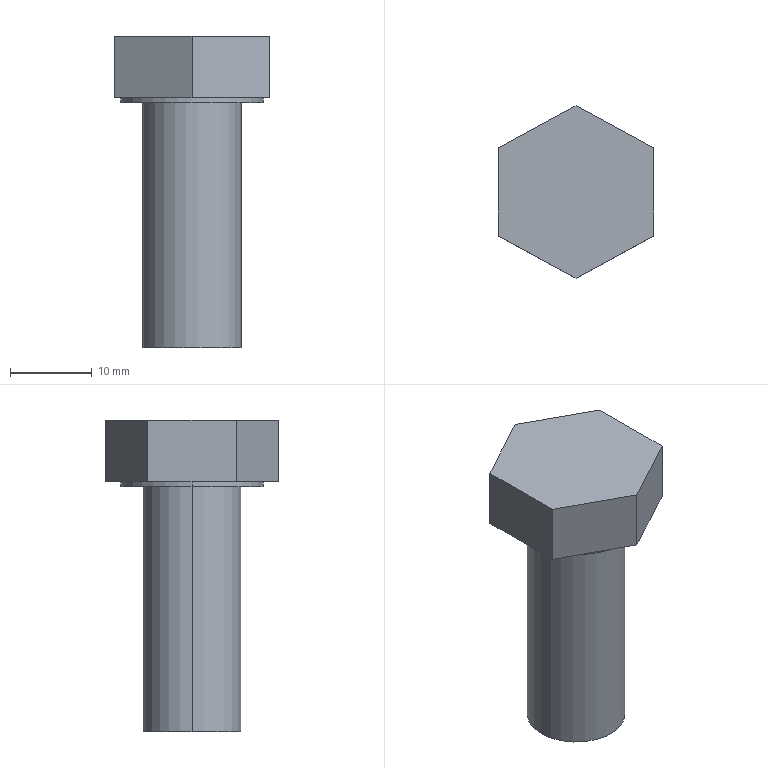Part | STEP file | M12-30 | 1 solid | 14 faces | box 19 x 21.1 x 38.1 mm | volume 5809 mm3 | plane 10 | cylinder 4 | commonest cylinder face diameters 12 x2 17.4 x2
STEP:
#1=CARTESIAN_POINT('',(0.,0.,0.));
#2=DIRECTION('',(0.,0.,1.));
#3=DIRECTION('',(1.,0.,0.));
#4=AXIS2_PLACEMENT_3D('',#1,#2,#3);
#5=CARTESIAN_POINT('',(0.,10.55,0.));
#6=VERTEX_POINT('',#5);
#7=CARTESIAN_POINT('',(-9.5,5.402,0.));
#8=VERTEX_POINT('',#7);
#9=CARTESIAN_POINT('',(0.,10.55,0.));
#10=DIRECTION('',(-0.8792,-0.4764,0.));
#11=VECTOR('',#10,1.);
#12=LINE('',#9,#11);
#13=CARTESIAN_POINT('',(0.,0.,0.));
#14=DIRECTION('',(0.,0.,1.));
#15=DIRECTION('',(1.,0.,0.));
#16=AXIS2_PLACEMENT_3D('',#13,#14,#15);
#17=PLANE('',#16);
#18=CARTESIAN_POINT('',(0.,10.55));
#19=DIRECTION('',(-0.8792,-0.4764));
#20=VECTOR('',#19,1.);
#21=LINE('',#18,#20);
#22=(GEOMETRIC_REPRESENTATION_CONTEXT(2)PARAMETRIC_REPRESENTATION_CONTEXT()REPRESENTATION_CONTEXT('',''));
#23=DEFINITIONAL_REPRESENTATION('',(#21),#22);
#24=PCURVE('',#17,#23);
#25=CARTESIAN_POINT('',(0.,10.55,0.));
#26=DIRECTION('',(-0.4764,0.8792,0.));
#27=DIRECTION('',(-0.8792,-0.4764,0.));
#28=AXIS2_PLACEMENT_3D('',#25,#26,#27);
#29=PLANE('',#28);
#30=CARTESIAN_POINT('',(0.,0.));
#31=DIRECTION('',(1.,0.));
#32=VECTOR('',#31,1.);
#33=LINE('',#30,#32);
#34=(GEOMETRIC_REPRESENTATION_CONTEXT(2)PARAMETRIC_REPRESENTATION_CONTEXT()REPRESENTATION_CONTEXT('',''));
#35=DEFINITIONAL_REPRESENTATION('',(#33),#34);
#36=PCURVE('',#29,#35);
#37=SURFACE_CURVE('',#12,(#24,#36),.PCURVE_S1.);
#38=EDGE_CURVE('',#6,#8,#37,.T.);
#39=ORIENTED_EDGE('',*,*,#38,.T.);
#40=CARTESIAN_POINT('',(-9.5,-5.402,0.));
#41=VERTEX_POINT('',#40);
#42=CARTESIAN_POINT('',(-9.5,5.402,0.));
#43=DIRECTION('',(0.,-1.,0.));
#44=VECTOR('',#43,1.);
#45=LINE('',#42,#44);
#46=CARTESIAN_POINT('',(-9.5,5.402));
#47=DIRECTION('',(0.,-1.));
#48=VECTOR('',#47,1.);
#49=LINE('',#46,#48);
#50=(GEOMETRIC_REPRESENTATION_CONTEXT(2)PARAMETRIC_REPRESENTATION_CONTEXT()REPRESENTATION_CONTEXT('',''));
#51=DEFINITIONAL_REPRESENTATION('',(#49),#50);
#52=PCURVE('',#17,#51);
#53=CARTESIAN_POINT('',(-9.5,5.402,0.));
#54=DIRECTION('',(-1.,0.,0.));
#55=DIRECTION('',(0.,-1.,0.));
#56=AXIS2_PLACEMENT_3D('',#53,#54,#55);
#57=PLANE('',#56);
#58=CARTESIAN_POINT('',(0.,0.));
#59=DIRECTION('',(1.,0.));
#60=VECTOR('',#59,1.);
#61=LINE('',#58,#60);
#62=(GEOMETRIC_REPRESENTATION_CONTEXT(2)PARAMETRIC_REPRESENTATION_CONTEXT()REPRESENTATION_CONTEXT('',''));
#63=DEFINITIONAL_REPRESENTATION('',(#61),#62);
#64=PCURVE('',#57,#63);
#65=SURFACE_CURVE('',#45,(#52,#64),.PCURVE_S1.);
#66=EDGE_CURVE('',#8,#41,#65,.T.);
#67=ORIENTED_EDGE('',*,*,#66,.T.);
#68=CARTESIAN_POINT('',(0.,-10.55,0.));
#69=VERTEX_POINT('',#68);
#70=CARTESIAN_POINT('',(-9.5,-5.402,0.));
#71=DIRECTION('',(0.8792,-0.4764,0.));
#72=VECTOR('',#71,1.);
#73=LINE('',#70,#72);
#74=CARTESIAN_POINT('',(-9.5,-5.402));
#75=DIRECTION('',(0.8792,-0.4764));
#76=VECTOR('',#75,1.);
#77=LINE('',#74,#76);
#78=(GEOMETRIC_REPRESENTATION_CONTEXT(2)PARAMETRIC_REPRESENTATION_CONTEXT()REPRESENTATION_CONTEXT('',''));
#79=DEFINITIONAL_REPRESENTATION('',(#77),#78);
#80=PCURVE('',#17,#79);
#81=CARTESIAN_POINT('',(-9.5,-5.402,0.));
#82=DIRECTION('',(-0.4764,-0.8792,0.));
#83=DIRECTION('',(0.8792,-0.4764,0.));
#84=AXIS2_PLACEMENT_3D('',#81,#82,#83);
#85=PLANE('',#84);
#86=CARTESIAN_POINT('',(0.,0.));
#87=DIRECTION('',(1.,0.));
#88=VECTOR('',#87,1.);
#89=LINE('',#86,#88);
#90=(GEOMETRIC_REPRESENTATION_CONTEXT(2)PARAMETRIC_REPRESENTATION_CONTEXT()REPRESENTATION_CONTEXT('',''));
#91=DEFINITIONAL_REPRESENTATION('',(#89),#90);
#92=PCURVE('',#85,#91);
#93=SURFACE_CURVE('',#73,(#80,#92),.PCURVE_S1.);
#94=EDGE_CURVE('',#41,#69,#93,.T.);
#95=ORIENTED_EDGE('',*,*,#94,.T.);
#96=CARTESIAN_POINT('',(9.5,-5.402,0.));
#97=VERTEX_POINT('',#96);
#98=CARTESIAN_POINT('',(0.,-10.55,0.));
#99=DIRECTION('',(0.8792,0.4764,0.));
#100=VECTOR('',#99,1.);
#101=LINE('',#98,#100);
#102=CARTESIAN_POINT('',(0.,-10.55));
#103=DIRECTION('',(0.8792,0.4764));
#104=VECTOR('',#103,1.);
#105=LINE('',#102,#104);
#106=(GEOMETRIC_REPRESENTATION_CONTEXT(2)PARAMETRIC_REPRESENTATION_CONTEXT()REPRESENTATION_CONTEXT('',''));
#107=DEFINITIONAL_REPRESENTATION('',(#105),#106);
#108=PCURVE('',#17,#107);
#109=CARTESIAN_POINT('',(0.,-10.55,0.));
#110=DIRECTION('',(0.4764,-0.8792,0.));
#111=DIRECTION('',(0.8792,0.4764,0.));
#112=AXIS2_PLACEMENT_3D('',#109,#110,#111);
#113=PLANE('',#112);
#114=CARTESIAN_POINT('',(0.,0.));
#115=DIRECTION('',(1.,0.));
#116=VECTOR('',#115,1.);
#117=LINE('',#114,#116);
#118=(GEOMETRIC_REPRESENTATION_CONTEXT(2)PARAMETRIC_REPRESENTATION_CONTEXT()REPRESENTATION_CONTEXT('',''));
#119=DEFINITIONAL_REPRESENTATION('',(#117),#118);
#120=PCURVE('',#113,#119);
#121=SURFACE_CURVE('',#101,(#108,#120),.PCURVE_S1.);
#122=EDGE_CURVE('',#69,#97,#121,.T.);
#123=ORIENTED_EDGE('',*,*,#122,.T.);
#124=CARTESIAN_POINT('',(9.5,5.402,0.));
#125=VERTEX_POINT('',#124);
#126=CARTESIAN_POINT('',(9.5,-5.402,0.));
#127=DIRECTION('',(0.,1.,0.));
#128=VECTOR('',#127,1.);
#129=LINE('',#126,#128);
#130=CARTESIAN_POINT('',(9.5,-5.402));
#131=DIRECTION('',(0.,1.));
#132=VECTOR('',#131,1.);
#133=LINE('',#130,#132);
#134=(GEOMETRIC_REPRESENTATION_CONTEXT(2)PARAMETRIC_REPRESENTATION_CONTEXT()REPRESENTATION_CONTEXT('',''));
#135=DEFINITIONAL_REPRESENTATION('',(#133),#134);
#136=PCURVE('',#17,#135);
#137=CARTESIAN_POINT('',(9.5,-5.402,0.));
#138=DIRECTION('',(1.,0.,0.));
#139=DIRECTION('',(0.,1.,0.));
#140=AXIS2_PLACEMENT_3D('',#137,#138,#139);
#141=PLANE('',#140);
#142=CARTESIAN_POINT('',(0.,0.));
#143=DIRECTION('',(1.,0.));
#144=VECTOR('',#143,1.);
#145=LINE('',#142,#144);
#146=(GEOMETRIC_REPRESENTATION_CONTEXT(2)PARAMETRIC_REPRESENTATION_CONTEXT()REPRESENTATION_CONTEXT('',''));
#147=DEFINITIONAL_REPRESENTATION('',(#145),#146);
#148=PCURVE('',#141,#147);
#149=SURFACE_CURVE('',#129,(#136,#148),.PCURVE_S1.);
#150=EDGE_CURVE('',#97,#125,#149,.T.);
#151=ORIENTED_EDGE('',*,*,#150,.T.);
#152=CARTESIAN_POINT('',(9.5,5.402,0.));
#153=DIRECTION('',(-0.8792,0.4764,0.));
#154=VECTOR('',#153,1.);
#155=LINE('',#152,#154);
#156=CARTESIAN_POINT('',(9.5,5.402));
#157=DIRECTION('',(-0.8792,0.4764));
#158=VECTOR('',#157,1.);
#159=LINE('',#156,#158);
#160=(GEOMETRIC_REPRESENTATION_CONTEXT(2)PARAMETRIC_REPRESENTATION_CONTEXT()REPRESENTATION_CONTEXT('',''));
#161=DEFINITIONAL_REPRESENTATION('',(#159),#160);
#162=PCURVE('',#17,#161);
#163=CARTESIAN_POINT('',(9.5,5.402,0.));
#164=DIRECTION('',(0.4764,0.8792,0.));
#165=DIRECTION('',(-0.8792,0.4764,0.));
#166=AXIS2_PLACEMENT_3D('',#163,#164,#165);
#167=PLANE('',#166);
#168=CARTESIAN_POINT('',(0.,0.));
#169=DIRECTION('',(1.,0.));
#170=VECTOR('',#169,1.);
#171=LINE('',#168,#170);
#172=(GEOMETRIC_REPRESENTATION_CONTEXT(2)PARAMETRIC_REPRESENTATION_CONTEXT()REPRESENTATION_CONTEXT('',''));
#173=DEFINITIONAL_REPRESENTATION('',(#171),#172);
#174=PCURVE('',#167,#173);
#175=SURFACE_CURVE('',#155,(#162,#174),.PCURVE_S1.);
#176=EDGE_CURVE('',#125,#6,#175,.T.);
#177=ORIENTED_EDGE('',*,*,#176,.T.);
#178=EDGE_LOOP('',(#39,#67,#95,#123,#151,#177));
#179=FACE_BOUND('',#178,.F.);
#180=CARTESIAN_POINT('',(-8.7,0.,0.));
#181=VERTEX_POINT('',#180);
#182=CARTESIAN_POINT('',(8.7,0.,0.));
#183=VERTEX_POINT('',#182);
#184=CARTESIAN_POINT('',(0.,0.,0.));
#185=DIRECTION('',(0.,0.,-1.));
#186=DIRECTION('',(-1.,0.,0.));
#187=AXIS2_PLACEMENT_3D('',#184,#185,#186);
#188=CIRCLE('',#187,8.7);
#189=CARTESIAN_POINT('',(-8.7,0.));
#190=CARTESIAN_POINT('',(-8.7,15.069));
#191=CARTESIAN_POINT('',(4.35,7.534));
#192=CARTESIAN_POINT('',(17.4,0.));
#193=CARTESIAN_POINT('',(4.35,-7.534));
#194=CARTESIAN_POINT('',(-8.7,-15.069));
#195=CARTESIAN_POINT('',(-8.7,0.));
#196=(BOUNDED_CURVE()B_SPLINE_CURVE(2,(#189,#190,#191,#192,#193,#194,#195),.UNSPECIFIED.,.T.,.F.)B_SPLINE_CURVE_WITH_KNOTS((1,2,2,2,2,1),(-2.094,0.,2.094,4.189,6.283,8.378),.UNSPECIFIED.)CURVE()GEOMETRIC_REPRESENTATION_ITEM()RATIONAL_B_SPLINE_CURVE((1.,0.5,1.,0.5,1.,0.5,1.))REPRESENTATION_ITEM(''));
#197=(GEOMETRIC_REPRESENTATION_CONTEXT(2)PARAMETRIC_REPRESENTATION_CONTEXT()REPRESENTATION_CONTEXT('',''));
#198=DEFINITIONAL_REPRESENTATION('',(#196),#197);
#199=PCURVE('',#17,#198);
#200=CARTESIAN_POINT('',(0.,0.,0.));
#201=DIRECTION('',(0.,0.,-1.));
#202=DIRECTION('',(-1.,0.,0.));
#203=AXIS2_PLACEMENT_3D('',#200,#201,#202);
#204=CYLINDRICAL_SURFACE('',#203,8.7);
#205=CARTESIAN_POINT('',(0.,0.));
#206=DIRECTION('',(1.,0.));
#207=VECTOR('',#206,1.);
#208=LINE('',#205,#207);
#209=(GEOMETRIC_REPRESENTATION_CONTEXT(2)PARAMETRIC_REPRESENTATION_CONTEXT()REPRESENTATION_CONTEXT('',''));
#210=DEFINITIONAL_REPRESENTATION('',(#208),#209);
#211=PCURVE('',#204,#210);
#212=SURFACE_CURVE('',#188,(#199,#211),.PCURVE_S1.);
#213=EDGE_CURVE('',#181,#183,#212,.T.);
#214=ORIENTED_EDGE('',*,*,#213,.T.);
#215=CARTESIAN_POINT('',(0.,0.,0.));
#216=DIRECTION('',(0.,0.,-1.));
#217=DIRECTION('',(1.,0.,0.));
#218=AXIS2_PLACEMENT_3D('',#215,#216,#217);
#219=CIRCLE('',#218,8.7);
#220=CARTESIAN_POINT('',(8.7,0.));
#221=CARTESIAN_POINT('',(8.7,-15.069));
#222=CARTESIAN_POINT('',(-4.35,-7.534));
#223=CARTESIAN_POINT('',(-17.4,0.));
#224=CARTESIAN_POINT('',(-4.35,7.534));
#225=CARTESIAN_POINT('',(8.7,15.069));
#226=CARTESIAN_POINT('',(8.7,0.));
#227=(BOUNDED_CURVE()B_SPLINE_CURVE(2,(#220,#221,#222,#223,#224,#225,#226),.UNSPECIFIED.,.T.,.F.)B_SPLINE_CURVE_WITH_KNOTS((1,2,2,2,2,1),(-2.094,0.,2.094,4.189,6.283,8.378),.UNSPECIFIED.)CURVE()GEOMETRIC_REPRESENTATION_ITEM()RATIONAL_B_SPLINE_CURVE((1.,0.5,1.,0.5,1.,0.5,1.))REPRESENTATION_ITEM(''));
#228=(GEOMETRIC_REPRESENTATION_CONTEXT(2)PARAMETRIC_REPRESENTATION_CONTEXT()REPRESENTATION_CONTEXT('',''));
#229=DEFINITIONAL_REPRESENTATION('',(#227),#228);
#230=PCURVE('',#17,#229);
#231=CARTESIAN_POINT('',(0.,0.,0.));
#232=DIRECTION('',(0.,0.,-1.));
#233=DIRECTION('',(-1.,0.,0.));
#234=AXIS2_PLACEMENT_3D('',#231,#232,#233);
#235=CYLINDRICAL_SURFACE('',#234,8.7);
#236=CARTESIAN_POINT('',(3.142,0.));
#237=DIRECTION('',(1.,0.));
#238=VECTOR('',#237,1.);
#239=LINE('',#236,#238);
#240=(GEOMETRIC_REPRESENTATION_CONTEXT(2)PARAMETRIC_REPRESENTATION_CONTEXT()REPRESENTATION_CONTEXT('',''));
#241=DEFINITIONAL_REPRESENTATION('',(#239),#240);
#242=PCURVE('',#235,#241);
#243=SURFACE_CURVE('',#219,(#230,#242),.PCURVE_S1.);
#244=EDGE_CURVE('',#183,#181,#243,.T.);
#245=ORIENTED_EDGE('',*,*,#244,.T.);
#246=EDGE_LOOP('',(#214,#245));
#247=FACE_BOUND('',#246,.F.);
#248=ADVANCED_FACE('',(#179,#247),#17,.F.);
#249=ORIENTED_EDGE('',*,*,#38,.F.);
#250=CARTESIAN_POINT('',(0.,10.55,7.5));
#251=VERTEX_POINT('',#250);
#252=CARTESIAN_POINT('',(0.,10.55,0.));
#253=DIRECTION('',(0.,0.,1.));
#254=VECTOR('',#253,1.);
#255=LINE('',#252,#254);
#256=CARTESIAN_POINT('',(0.,0.));
#257=DIRECTION('',(0.,1.));
#258=VECTOR('',#257,1.);
#259=LINE('',#256,#258);
#260=(GEOMETRIC_REPRESENTATION_CONTEXT(2)PARAMETRIC_REPRESENTATION_CONTEXT()REPRESENTATION_CONTEXT('',''));
#261=DEFINITIONAL_REPRESENTATION('',(#259),#260);
#262=PCURVE('',#29,#261);
#263=CARTESIAN_POINT('',(10.805,0.));
#264=DIRECTION('',(0.,1.));
#265=VECTOR('',#264,1.);
#266=LINE('',#263,#265);
#267=(GEOMETRIC_REPRESENTATION_CONTEXT(2)PARAMETRIC_REPRESENTATION_CONTEXT()REPRESENTATION_CONTEXT('',''));
#268=DEFINITIONAL_REPRESENTATION('',(#266),#267);
#269=PCURVE('',#167,#268);
#270=SURFACE_CURVE('',#255,(#262,#269),.PCURVE_S1.);
#271=EDGE_CURVE('',#6,#251,#270,.T.);
#272=ORIENTED_EDGE('',*,*,#271,.T.);
#273=CARTESIAN_POINT('',(-9.5,5.402,7.5));
#274=VERTEX_POINT('',#273);
#275=CARTESIAN_POINT('',(0.,10.55,7.5));
#276=DIRECTION('',(-0.8792,-0.4764,0.));
#277=VECTOR('',#276,1.);
#278=LINE('',#275,#277);
#279=CARTESIAN_POINT('',(0.,7.5));
#280=DIRECTION('',(1.,0.));
#281=VECTOR('',#280,1.);
#282=LINE('',#279,#281);
#283=(GEOMETRIC_REPRESENTATION_CONTEXT(2)PARAMETRIC_REPRESENTATION_CONTEXT()REPRESENTATION_CONTEXT('',''));
#284=DEFINITIONAL_REPRESENTATION('',(#282),#283);
#285=PCURVE('',#29,#284);
#286=CARTESIAN_POINT('',(0.,0.,7.5));
#287=DIRECTION('',(0.,0.,1.));
#288=DIRECTION('',(1.,0.,0.));
#289=AXIS2_PLACEMENT_3D('',#286,#287,#288);
#290=PLANE('',#289);
#291=CARTESIAN_POINT('',(0.,10.55));
#292=DIRECTION('',(-0.8792,-0.4764));
#293=VECTOR('',#292,1.);
#294=LINE('',#291,#293);
#295=(GEOMETRIC_REPRESENTATION_CONTEXT(2)PARAMETRIC_REPRESENTATION_CONTEXT()REPRESENTATION_CONTEXT('',''));
#296=DEFINITIONAL_REPRESENTATION('',(#294),#295);
#297=PCURVE('',#290,#296);
#298=SURFACE_CURVE('',#278,(#285,#297),.PCURVE_S1.);
#299=EDGE_CURVE('',#251,#274,#298,.T.);
#300=ORIENTED_EDGE('',*,*,#299,.T.);
#301=CARTESIAN_POINT('',(-9.5,5.402,0.));
#302=DIRECTION('',(0.,0.,1.));
#303=VECTOR('',#302,1.);
#304=LINE('',#301,#303);
#305=CARTESIAN_POINT('',(10.805,0.));
#306=DIRECTION('',(0.,1.));
#307=VECTOR('',#306,1.);
#308=LINE('',#305,#307);
#309=(GEOMETRIC_REPRESENTATION_CONTEXT(2)PARAMETRIC_REPRESENTATION_CONTEXT()REPRESENTATION_CONTEXT('',''));
#310=DEFINITIONAL_REPRESENTATION('',(#308),#309);
#311=PCURVE('',#29,#310);
#312=CARTESIAN_POINT('',(0.,0.));
#313=DIRECTION('',(0.,1.));
#314=VECTOR('',#313,1.);
#315=LINE('',#312,#314);
#316=(GEOMETRIC_REPRESENTATION_CONTEXT(2)PARAMETRIC_REPRESENTATION_CONTEXT()REPRESENTATION_CONTEXT('',''));
#317=DEFINITIONAL_REPRESENTATION('',(#315),#316);
#318=PCURVE('',#57,#317);
#319=SURFACE_CURVE('',#304,(#311,#318),.PCURVE_S1.);
#320=EDGE_CURVE('',#8,#274,#319,.T.);
#321=ORIENTED_EDGE('',*,*,#320,.F.);
#322=EDGE_LOOP('',(#249,#272,#300,#321));
#323=FACE_BOUND('',#322,.F.);
#324=ADVANCED_FACE('',(#323),#29,.T.);
#325=ORIENTED_EDGE('',*,*,#176,.F.);
#326=CARTESIAN_POINT('',(9.5,5.402,7.5));
#327=VERTEX_POINT('',#326);
#328=CARTESIAN_POINT('',(9.5,5.402,0.));
#329=DIRECTION('',(0.,0.,1.));
#330=VECTOR('',#329,1.);
#331=LINE('',#328,#330);
#332=CARTESIAN_POINT('',(0.,0.));
#333=DIRECTION('',(0.,1.));
#334=VECTOR('',#333,1.);
#335=LINE('',#332,#334);
#336=(GEOMETRIC_REPRESENTATION_CONTEXT(2)PARAMETRIC_REPRESENTATION_CONTEXT()REPRESENTATION_CONTEXT('',''));
#337=DEFINITIONAL_REPRESENTATION('',(#335),#336);
#338=PCURVE('',#167,#337);
#339=CARTESIAN_POINT('',(10.805,0.));
#340=DIRECTION('',(0.,1.));
#341=VECTOR('',#340,1.);
#342=LINE('',#339,#341);
#343=(GEOMETRIC_REPRESENTATION_CONTEXT(2)PARAMETRIC_REPRESENTATION_CONTEXT()REPRESENTATION_CONTEXT('',''));
#344=DEFINITIONAL_REPRESENTATION('',(#342),#343);
#345=PCURVE('',#141,#344);
#346=SURFACE_CURVE('',#331,(#338,#345),.PCURVE_S1.);
#347=EDGE_CURVE('',#125,#327,#346,.T.);
#348=ORIENTED_EDGE('',*,*,#347,.T.);
#349=CARTESIAN_POINT('',(9.5,5.402,7.5));
#350=DIRECTION('',(-0.8792,0.4764,0.));
#351=VECTOR('',#350,1.);
#352=LINE('',#349,#351);
#353=CARTESIAN_POINT('',(0.,7.5));
#354=DIRECTION('',(1.,0.));
#355=VECTOR('',#354,1.);
#356=LINE('',#353,#355);
#357=(GEOMETRIC_REPRESENTATION_CONTEXT(2)PARAMETRIC_REPRESENTATION_CONTEXT()REPRESENTATION_CONTEXT('',''));
#358=DEFINITIONAL_REPRESENTATION('',(#356),#357);
#359=PCURVE('',#167,#358);
#360=CARTESIAN_POINT('',(9.5,5.402));
#361=DIRECTION('',(-0.8792,0.4764));
#362=VECTOR('',#361,1.);
#363=LINE('',#360,#362);
#364=(GEOMETRIC_REPRESENTATION_CONTEXT(2)PARAMETRIC_REPRESENTATION_CONTEXT()REPRESENTATION_CONTEXT('',''));
#365=DEFINITIONAL_REPRESENTATION('',(#363),#364);
#366=PCURVE('',#290,#365);
#367=SURFACE_CURVE('',#352,(#359,#366),.PCURVE_S1.);
#368=EDGE_CURVE('',#327,#251,#367,.T.);
#369=ORIENTED_EDGE('',*,*,#368,.T.);
#370=ORIENTED_EDGE('',*,*,#271,.F.);
#371=EDGE_LOOP('',(#325,#348,#369,#370));
#372=FACE_BOUND('',#371,.F.);
#373=ADVANCED_FACE('',(#372),#167,.T.);
#374=ORIENTED_EDGE('',*,*,#150,.F.);
#375=CARTESIAN_POINT('',(9.5,-5.402,7.5));
#376=VERTEX_POINT('',#375);
#377=CARTESIAN_POINT('',(9.5,-5.402,0.));
#378=DIRECTION('',(0.,0.,1.));
#379=VECTOR('',#378,1.);
#380=LINE('',#377,#379);
#381=CARTESIAN_POINT('',(0.,0.));
#382=DIRECTION('',(0.,1.));
#383=VECTOR('',#382,1.);
#384=LINE('',#381,#383);
#385=(GEOMETRIC_REPRESENTATION_CONTEXT(2)PARAMETRIC_REPRESENTATION_CONTEXT()REPRESENTATION_CONTEXT('',''));
#386=DEFINITIONAL_REPRESENTATION('',(#384),#385);
#387=PCURVE('',#141,#386);
#388=CARTESIAN_POINT('',(10.805,0.));
#389=DIRECTION('',(0.,1.));
#390=VECTOR('',#389,1.);
#391=LINE('',#388,#390);
#392=(GEOMETRIC_REPRESENTATION_CONTEXT(2)PARAMETRIC_REPRESENTATION_CONTEXT()REPRESENTATION_CONTEXT('',''));
#393=DEFINITIONAL_REPRESENTATION('',(#391),#392);
#394=PCURVE('',#113,#393);
#395=SURFACE_CURVE('',#380,(#387,#394),.PCURVE_S1.);
#396=EDGE_CURVE('',#97,#376,#395,.T.);
#397=ORIENTED_EDGE('',*,*,#396,.T.);
#398=CARTESIAN_POINT('',(9.5,-5.402,7.5));
#399=DIRECTION('',(0.,1.,0.));
#400=VECTOR('',#399,1.);
#401=LINE('',#398,#400);
#402=CARTESIAN_POINT('',(0.,7.5));
#403=DIRECTION('',(1.,0.));
#404=VECTOR('',#403,1.);
#405=LINE('',#402,#404);
#406=(GEOMETRIC_REPRESENTATION_CONTEXT(2)PARAMETRIC_REPRESENTATION_CONTEXT()REPRESENTATION_CONTEXT('',''));
#407=DEFINITIONAL_REPRESENTATION('',(#405),#406);
#408=PCURVE('',#141,#407);
#409=CARTESIAN_POINT('',(9.5,-5.402));
#410=DIRECTION('',(0.,1.));
#411=VECTOR('',#410,1.);
#412=LINE('',#409,#411);
#413=(GEOMETRIC_REPRESENTATION_CONTEXT(2)PARAMETRIC_REPRESENTATION_CONTEXT()REPRESENTATION_CONTEXT('',''));
#414=DEFINITIONAL_REPRESENTATION('',(#412),#413);
#415=PCURVE('',#290,#414);
#416=SURFACE_CURVE('',#401,(#408,#415),.PCURVE_S1.);
#417=EDGE_CURVE('',#376,#327,#416,.T.);
#418=ORIENTED_EDGE('',*,*,#417,.T.);
#419=ORIENTED_EDGE('',*,*,#347,.F.);
#420=EDGE_LOOP('',(#374,#397,#418,#419));
#421=FACE_BOUND('',#420,.F.);
#422=ADVANCED_FACE('',(#421),#141,.T.);
#423=ORIENTED_EDGE('',*,*,#122,.F.);
#424=CARTESIAN_POINT('',(0.,-10.55,7.5));
#425=VERTEX_POINT('',#424);
#426=CARTESIAN_POINT('',(0.,-10.55,0.));
#427=DIRECTION('',(0.,0.,1.));
#428=VECTOR('',#427,1.);
#429=LINE('',#426,#428);
#430=CARTESIAN_POINT('',(0.,0.));
#431=DIRECTION('',(0.,1.));
#432=VECTOR('',#431,1.);
#433=LINE('',#430,#432);
#434=(GEOMETRIC_REPRESENTATION_CONTEXT(2)PARAMETRIC_REPRESENTATION_CONTEXT()REPRESENTATION_CONTEXT('',''));
#435=DEFINITIONAL_REPRESENTATION('',(#433),#434);
#436=PCURVE('',#113,#435);
#437=CARTESIAN_POINT('',(10.805,0.));
#438=DIRECTION('',(0.,1.));
#439=VECTOR('',#438,1.);
#440=LINE('',#437,#439);
#441=(GEOMETRIC_REPRESENTATION_CONTEXT(2)PARAMETRIC_REPRESENTATION_CONTEXT()REPRESENTATION_CONTEXT('',''));
#442=DEFINITIONAL_REPRESENTATION('',(#440),#441);
#443=PCURVE('',#85,#442);
#444=SURFACE_CURVE('',#429,(#436,#443),.PCURVE_S1.);
#445=EDGE_CURVE('',#69,#425,#444,.T.);
#446=ORIENTED_EDGE('',*,*,#445,.T.);
#447=CARTESIAN_POINT('',(0.,-10.55,7.5));
#448=DIRECTION('',(0.8792,0.4764,0.));
#449=VECTOR('',#448,1.);
#450=LINE('',#447,#449);
#451=CARTESIAN_POINT('',(0.,7.5));
#452=DIRECTION('',(1.,0.));
#453=VECTOR('',#452,1.);
#454=LINE('',#451,#453);
#455=(GEOMETRIC_REPRESENTATION_CONTEXT(2)PARAMETRIC_REPRESENTATION_CONTEXT()REPRESENTATION_CONTEXT('',''));
#456=DEFINITIONAL_REPRESENTATION('',(#454),#455);
#457=PCURVE('',#113,#456);
#458=CARTESIAN_POINT('',(0.,-10.55));
#459=DIRECTION('',(0.8792,0.4764));
#460=VECTOR('',#459,1.);
#461=LINE('',#458,#460);
#462=(GEOMETRIC_REPRESENTATION_CONTEXT(2)PARAMETRIC_REPRESENTATION_CONTEXT()REPRESENTATION_CONTEXT('',''));
#463=DEFINITIONAL_REPRESENTATION('',(#461),#462);
#464=PCURVE('',#290,#463);
#465=SURFACE_CURVE('',#450,(#457,#464),.PCURVE_S1.);
#466=EDGE_CURVE('',#425,#376,#465,.T.);
#467=ORIENTED_EDGE('',*,*,#466,.T.);
#468=ORIENTED_EDGE('',*,*,#396,.F.);
#469=EDGE_LOOP('',(#423,#446,#467,#468));
#470=FACE_BOUND('',#469,.F.);
#471=ADVANCED_FACE('',(#470),#113,.T.);
#472=ORIENTED_EDGE('',*,*,#94,.F.);
#473=CARTESIAN_POINT('',(-9.5,-5.402,7.5));
#474=VERTEX_POINT('',#473);
#475=CARTESIAN_POINT('',(-9.5,-5.402,0.));
#476=DIRECTION('',(0.,0.,1.));
#477=VECTOR('',#476,1.);
#478=LINE('',#475,#477);
#479=CARTESIAN_POINT('',(0.,0.));
#480=DIRECTION('',(0.,1.));
#481=VECTOR('',#480,1.);
#482=LINE('',#479,#481);
#483=(GEOMETRIC_REPRESENTATION_CONTEXT(2)PARAMETRIC_REPRESENTATION_CONTEXT()REPRESENTATION_CONTEXT('',''));
#484=DEFINITIONAL_REPRESENTATION('',(#482),#483);
#485=PCURVE('',#85,#484);
#486=CARTESIAN_POINT('',(10.805,0.));
#487=DIRECTION('',(0.,1.));
#488=VECTOR('',#487,1.);
#489=LINE('',#486,#488);
#490=(GEOMETRIC_REPRESENTATION_CONTEXT(2)PARAMETRIC_REPRESENTATION_CONTEXT()REPRESENTATION_CONTEXT('',''));
#491=DEFINITIONAL_REPRESENTATION('',(#489),#490);
#492=PCURVE('',#57,#491);
#493=SURFACE_CURVE('',#478,(#485,#492),.PCURVE_S1.);
#494=EDGE_CURVE('',#41,#474,#493,.T.);
#495=ORIENTED_EDGE('',*,*,#494,.T.);
#496=CARTESIAN_POINT('',(-9.5,-5.402,7.5));
#497=DIRECTION('',(0.8792,-0.4764,0.));
#498=VECTOR('',#497,1.);
#499=LINE('',#496,#498);
#500=CARTESIAN_POINT('',(0.,7.5));
#501=DIRECTION('',(1.,0.));
#502=VECTOR('',#501,1.);
#503=LINE('',#500,#502);
#504=(GEOMETRIC_REPRESENTATION_CONTEXT(2)PARAMETRIC_REPRESENTATION_CONTEXT()REPRESENTATION_CONTEXT('',''));
#505=DEFINITIONAL_REPRESENTATION('',(#503),#504);
#506=PCURVE('',#85,#505);
#507=CARTESIAN_POINT('',(-9.5,-5.402));
#508=DIRECTION('',(0.8792,-0.4764));
#509=VECTOR('',#508,1.);
#510=LINE('',#507,#509);
#511=(GEOMETRIC_REPRESENTATION_CONTEXT(2)PARAMETRIC_REPRESENTATION_CONTEXT()REPRESENTATION_CONTEXT('',''));
#512=DEFINITIONAL_REPRESENTATION('',(#510),#511);
#513=PCURVE('',#290,#512);
#514=SURFACE_CURVE('',#499,(#506,#513),.PCURVE_S1.);
#515=EDGE_CURVE('',#474,#425,#514,.T.);
#516=ORIENTED_EDGE('',*,*,#515,.T.);
#517=ORIENTED_EDGE('',*,*,#445,.F.);
#518=EDGE_LOOP('',(#472,#495,#516,#517));
#519=FACE_BOUND('',#518,.F.);
#520=ADVANCED_FACE('',(#519),#85,.T.);
#521=ORIENTED_EDGE('',*,*,#66,.F.);
#522=ORIENTED_EDGE('',*,*,#320,.T.);
#523=CARTESIAN_POINT('',(-9.5,5.402,7.5));
#524=DIRECTION('',(0.,-1.,0.));
#525=VECTOR('',#524,1.);
#526=LINE('',#523,#525);
#527=CARTESIAN_POINT('',(0.,7.5));
#528=DIRECTION('',(1.,0.));
#529=VECTOR('',#528,1.);
#530=LINE('',#527,#529);
#531=(GEOMETRIC_REPRESENTATION_CONTEXT(2)PARAMETRIC_REPRESENTATION_CONTEXT()REPRESENTATION_CONTEXT('',''));
#532=DEFINITIONAL_REPRESENTATION('',(#530),#531);
#533=PCURVE('',#57,#532);
#534=CARTESIAN_POINT('',(-9.5,5.402));
#535=DIRECTION('',(0.,-1.));
#536=VECTOR('',#535,1.);
#537=LINE('',#534,#536);
#538=(GEOMETRIC_REPRESENTATION_CONTEXT(2)PARAMETRIC_REPRESENTATION_CONTEXT()REPRESENTATION_CONTEXT('',''));
#539=DEFINITIONAL_REPRESENTATION('',(#537),#538);
#540=PCURVE('',#290,#539);
#541=SURFACE_CURVE('',#526,(#533,#540),.PCURVE_S1.);
#542=EDGE_CURVE('',#274,#474,#541,.T.);
#543=ORIENTED_EDGE('',*,*,#542,.T.);
#544=ORIENTED_EDGE('',*,*,#494,.F.);
#545=EDGE_LOOP('',(#521,#522,#543,#544));
#546=FACE_BOUND('',#545,.F.);
#547=ADVANCED_FACE('',(#546),#57,.T.);
#548=ORIENTED_EDGE('',*,*,#299,.F.);
#549=ORIENTED_EDGE('',*,*,#368,.F.);
#550=ORIENTED_EDGE('',*,*,#417,.F.);
#551=ORIENTED_EDGE('',*,*,#466,.F.);
#552=ORIENTED_EDGE('',*,*,#515,.F.);
#553=ORIENTED_EDGE('',*,*,#542,.F.);
#554=EDGE_LOOP('',(#548,#549,#550,#551,#552,#553));
#555=FACE_BOUND('',#554,.F.);
#556=ADVANCED_FACE('',(#555),#290,.T.);
#557=CARTESIAN_POINT('',(8.7,0.,-0.6));
#558=VERTEX_POINT('',#557);
#559=CARTESIAN_POINT('',(8.7,0.,0.));
#560=DIRECTION('',(0.,0.,-1.));
#561=VECTOR('',#560,1.);
#562=LINE('',#559,#561);
#563=CARTESIAN_POINT('',(3.142,0.));
#564=DIRECTION('',(0.,1.));
#565=VECTOR('',#564,1.);
#566=LINE('',#563,#565);
#567=(GEOMETRIC_REPRESENTATION_CONTEXT(2)PARAMETRIC_REPRESENTATION_CONTEXT()REPRESENTATION_CONTEXT('',''));
#568=DEFINITIONAL_REPRESENTATION('',(#566),#567);
#569=PCURVE('',#204,#568);
#570=CARTESIAN_POINT('',(3.142,0.));
#571=DIRECTION('',(0.,1.));
#572=VECTOR('',#571,1.);
#573=LINE('',#570,#572);
#574=(GEOMETRIC_REPRESENTATION_CONTEXT(2)PARAMETRIC_REPRESENTATION_CONTEXT()REPRESENTATION_CONTEXT('',''));
#575=DEFINITIONAL_REPRESENTATION('',(#573),#574);
#576=PCURVE('',#235,#575);
#577=SURFACE_CURVE('',#562,(#569,#576),.PCURVE_S1.);
#578=EDGE_CURVE('',#183,#558,#577,.T.);
#579=ORIENTED_EDGE('',*,*,#578,.T.);
#580=CARTESIAN_POINT('',(-8.7,0.,-0.6));
#581=VERTEX_POINT('',#580);
#582=CARTESIAN_POINT('',(0.,0.,-0.6));
#583=DIRECTION('',(0.,0.,-1.));
#584=DIRECTION('',(-1.,0.,0.));
#585=AXIS2_PLACEMENT_3D('',#582,#583,#584);
#586=CIRCLE('',#585,8.7);
#587=CARTESIAN_POINT('',(0.,0.6));
#588=DIRECTION('',(1.,0.));
#589=VECTOR('',#588,1.);
#590=LINE('',#587,#589);
#591=(GEOMETRIC_REPRESENTATION_CONTEXT(2)PARAMETRIC_REPRESENTATION_CONTEXT()REPRESENTATION_CONTEXT('',''));
#592=DEFINITIONAL_REPRESENTATION('',(#590),#591);
#593=PCURVE('',#204,#592);
#594=CARTESIAN_POINT('',(0.,0.,-0.6));
#595=DIRECTION('',(0.,0.,-1.));
#596=DIRECTION('',(-1.,0.,0.));
#597=AXIS2_PLACEMENT_3D('',#594,#595,#596);
#598=PLANE('',#597);
#599=CARTESIAN_POINT('',(0.,0.));
#600=DIRECTION('',(1.,0.));
#601=AXIS2_PLACEMENT_2D('',#599,#600);
#602=CIRCLE('',#601,8.7);
#603=(GEOMETRIC_REPRESENTATION_CONTEXT(2)PARAMETRIC_REPRESENTATION_CONTEXT()REPRESENTATION_CONTEXT('',''));
#604=DEFINITIONAL_REPRESENTATION('',(#602),#603);
#605=PCURVE('',#598,#604);
#606=SURFACE_CURVE('',#586,(#593,#605),.PCURVE_S1.);
#607=EDGE_CURVE('',#581,#558,#606,.T.);
#608=ORIENTED_EDGE('',*,*,#607,.F.);
#609=CARTESIAN_POINT('',(-8.7,0.,0.));
#610=DIRECTION('',(0.,0.,-1.));
#611=VECTOR('',#610,1.);
#612=LINE('',#609,#611);
#613=CARTESIAN_POINT('',(0.,0.));
#614=DIRECTION('',(0.,1.));
#615=VECTOR('',#614,1.);
#616=LINE('',#613,#615);
#617=(GEOMETRIC_REPRESENTATION_CONTEXT(2)PARAMETRIC_REPRESENTATION_CONTEXT()REPRESENTATION_CONTEXT('',''));
#618=DEFINITIONAL_REPRESENTATION('',(#616),#617);
#619=PCURVE('',#204,#618);
#620=CARTESIAN_POINT('',(6.283,0.));
#621=DIRECTION('',(0.,1.));
#622=VECTOR('',#621,1.);
#623=LINE('',#620,#622);
#624=(GEOMETRIC_REPRESENTATION_CONTEXT(2)PARAMETRIC_REPRESENTATION_CONTEXT()REPRESENTATION_CONTEXT('',''));
#625=DEFINITIONAL_REPRESENTATION('',(#623),#624);
#626=PCURVE('',#235,#625);
#627=SURFACE_CURVE('',#612,(#619,#626),.PCURVE_S1.);
#628=EDGE_CURVE('',#181,#581,#627,.T.);
#629=ORIENTED_EDGE('',*,*,#628,.F.);
#630=ORIENTED_EDGE('',*,*,#213,.T.);
#631=EDGE_LOOP('',(#579,#608,#629,#630));
#632=FACE_BOUND('',#631,.T.);
#633=ADVANCED_FACE('',(#632),#204,.T.);
#634=ORIENTED_EDGE('',*,*,#628,.T.);
#635=CARTESIAN_POINT('',(0.,0.,-0.6));
#636=DIRECTION('',(0.,0.,-1.));
#637=DIRECTION('',(1.,0.,0.));
#638=AXIS2_PLACEMENT_3D('',#635,#636,#637);
#639=CIRCLE('',#638,8.7);
#640=CARTESIAN_POINT('',(3.142,0.6));
#641=DIRECTION('',(1.,0.));
#642=VECTOR('',#641,1.);
#643=LINE('',#640,#642);
#644=(GEOMETRIC_REPRESENTATION_CONTEXT(2)PARAMETRIC_REPRESENTATION_CONTEXT()REPRESENTATION_CONTEXT('',''));
#645=DEFINITIONAL_REPRESENTATION('',(#643),#644);
#646=PCURVE('',#235,#645);
#647=CARTESIAN_POINT('',(0.,0.));
#648=DIRECTION('',(-1.,0.));
#649=AXIS2_PLACEMENT_2D('',#647,#648);
#650=CIRCLE('',#649,8.7);
#651=(GEOMETRIC_REPRESENTATION_CONTEXT(2)PARAMETRIC_REPRESENTATION_CONTEXT()REPRESENTATION_CONTEXT('',''));
#652=DEFINITIONAL_REPRESENTATION('',(#650),#651);
#653=PCURVE('',#598,#652);
#654=SURFACE_CURVE('',#639,(#646,#653),.PCURVE_S1.);
#655=EDGE_CURVE('',#558,#581,#654,.T.);
#656=ORIENTED_EDGE('',*,*,#655,.F.);
#657=ORIENTED_EDGE('',*,*,#578,.F.);
#658=ORIENTED_EDGE('',*,*,#244,.T.);
#659=EDGE_LOOP('',(#634,#656,#657,#658));
#660=FACE_BOUND('',#659,.T.);
#661=ADVANCED_FACE('',(#660),#235,.T.);
#662=ORIENTED_EDGE('',*,*,#607,.F.);
#663=ORIENTED_EDGE('',*,*,#655,.F.);
#664=EDGE_LOOP('',(#662,#663));
#665=FACE_BOUND('',#664,.F.);
#666=CARTESIAN_POINT('',(-6.,0.,-0.6));
#667=VERTEX_POINT('',#666);
#668=CARTESIAN_POINT('',(6.,0.,-0.6));
#669=VERTEX_POINT('',#668);
#670=CARTESIAN_POINT('',(0.,0.,-0.6));
#671=DIRECTION('',(0.,0.,-1.));
#672=DIRECTION('',(-1.,0.,0.));
#673=AXIS2_PLACEMENT_3D('',#670,#671,#672);
#674=CIRCLE('',#673,6.);
#675=CARTESIAN_POINT('',(0.,0.));
#676=DIRECTION('',(1.,0.));
#677=AXIS2_PLACEMENT_2D('',#675,#676);
#678=CIRCLE('',#677,6.);
#679=(GEOMETRIC_REPRESENTATION_CONTEXT(2)PARAMETRIC_REPRESENTATION_CONTEXT()REPRESENTATION_CONTEXT('',''));
#680=DEFINITIONAL_REPRESENTATION('',(#678),#679);
#681=PCURVE('',#598,#680);
#682=CARTESIAN_POINT('',(0.,0.,-0.6));
#683=DIRECTION('',(0.,0.,-1.));
#684=DIRECTION('',(-1.,0.,0.));
#685=AXIS2_PLACEMENT_3D('',#682,#683,#684);
#686=CYLINDRICAL_SURFACE('',#685,6.);
#687=CARTESIAN_POINT('',(0.,0.));
#688=DIRECTION('',(1.,0.));
#689=VECTOR('',#688,1.);
#690=LINE('',#687,#689);
#691=(GEOMETRIC_REPRESENTATION_CONTEXT(2)PARAMETRIC_REPRESENTATION_CONTEXT()REPRESENTATION_CONTEXT('',''));
#692=DEFINITIONAL_REPRESENTATION('',(#690),#691);
#693=PCURVE('',#686,#692);
#694=SURFACE_CURVE('',#674,(#681,#693),.PCURVE_S1.);
#695=EDGE_CURVE('',#667,#669,#694,.T.);
#696=ORIENTED_EDGE('',*,*,#695,.T.);
#697=CARTESIAN_POINT('',(0.,0.,-0.6));
#698=DIRECTION('',(0.,0.,-1.));
#699=DIRECTION('',(1.,0.,0.));
#700=AXIS2_PLACEMENT_3D('',#697,#698,#699);
#701=CIRCLE('',#700,6.);
#702=CARTESIAN_POINT('',(0.,0.));
#703=DIRECTION('',(-1.,0.));
#704=AXIS2_PLACEMENT_2D('',#702,#703);
#705=CIRCLE('',#704,6.);
#706=(GEOMETRIC_REPRESENTATION_CONTEXT(2)PARAMETRIC_REPRESENTATION_CONTEXT()REPRESENTATION_CONTEXT('',''));
#707=DEFINITIONAL_REPRESENTATION('',(#705),#706);
#708=PCURVE('',#598,#707);
#709=CARTESIAN_POINT('',(0.,0.,-0.6));
#710=DIRECTION('',(0.,0.,-1.));
#711=DIRECTION('',(-1.,0.,0.));
#712=AXIS2_PLACEMENT_3D('',#709,#710,#711);
#713=CYLINDRICAL_SURFACE('',#712,6.);
#714=CARTESIAN_POINT('',(3.142,0.));
#715=DIRECTION('',(1.,0.));
#716=VECTOR('',#715,1.);
#717=LINE('',#714,#716);
#718=(GEOMETRIC_REPRESENTATION_CONTEXT(2)PARAMETRIC_REPRESENTATION_CONTEXT()REPRESENTATION_CONTEXT('',''));
#719=DEFINITIONAL_REPRESENTATION('',(#717),#718);
#720=PCURVE('',#713,#719);
#721=SURFACE_CURVE('',#701,(#708,#720),.PCURVE_S1.);
#722=EDGE_CURVE('',#669,#667,#721,.T.);
#723=ORIENTED_EDGE('',*,*,#722,.T.);
#724=EDGE_LOOP('',(#696,#723));
#725=FACE_BOUND('',#724,.F.);
#726=ADVANCED_FACE('',(#665,#725),#598,.T.);
#727=CARTESIAN_POINT('',(6.,0.,-30.6));
#728=VERTEX_POINT('',#727);
#729=CARTESIAN_POINT('',(6.,0.,-0.6));
#730=DIRECTION('',(0.,0.,-1.));
#731=VECTOR('',#730,1.);
#732=LINE('',#729,#731);
#733=CARTESIAN_POINT('',(3.142,0.));
#734=DIRECTION('',(0.,1.));
#735=VECTOR('',#734,1.);
#736=LINE('',#733,#735);
#737=(GEOMETRIC_REPRESENTATION_CONTEXT(2)PARAMETRIC_REPRESENTATION_CONTEXT()REPRESENTATION_CONTEXT('',''));
#738=DEFINITIONAL_REPRESENTATION('',(#736),#737);
#739=PCURVE('',#686,#738);
#740=CARTESIAN_POINT('',(3.142,0.));
#741=DIRECTION('',(0.,1.));
#742=VECTOR('',#741,1.);
#743=LINE('',#740,#742);
#744=(GEOMETRIC_REPRESENTATION_CONTEXT(2)PARAMETRIC_REPRESENTATION_CONTEXT()REPRESENTATION_CONTEXT('',''));
#745=DEFINITIONAL_REPRESENTATION('',(#743),#744);
#746=PCURVE('',#713,#745);
#747=SURFACE_CURVE('',#732,(#739,#746),.PCURVE_S1.);
#748=EDGE_CURVE('',#669,#728,#747,.T.);
#749=ORIENTED_EDGE('',*,*,#748,.T.);
#750=CARTESIAN_POINT('',(-6.,0.,-30.6));
#751=VERTEX_POINT('',#750);
#752=CARTESIAN_POINT('',(0.,0.,-30.6));
#753=DIRECTION('',(0.,0.,-1.));
#754=DIRECTION('',(-1.,0.,0.));
#755=AXIS2_PLACEMENT_3D('',#752,#753,#754);
#756=CIRCLE('',#755,6.);
#757=CARTESIAN_POINT('',(0.,30.));
#758=DIRECTION('',(1.,0.));
#759=VECTOR('',#758,1.);
#760=LINE('',#757,#759);
#761=(GEOMETRIC_REPRESENTATION_CONTEXT(2)PARAMETRIC_REPRESENTATION_CONTEXT()REPRESENTATION_CONTEXT('',''));
#762=DEFINITIONAL_REPRESENTATION('',(#760),#761);
#763=PCURVE('',#686,#762);
#764=CARTESIAN_POINT('',(0.,0.,-30.6));
#765=DIRECTION('',(0.,0.,-1.));
#766=DIRECTION('',(-1.,0.,0.));
#767=AXIS2_PLACEMENT_3D('',#764,#765,#766);
#768=PLANE('',#767);
#769=CARTESIAN_POINT('',(0.,0.));
#770=DIRECTION('',(1.,0.));
#771=AXIS2_PLACEMENT_2D('',#769,#770);
#772=CIRCLE('',#771,6.);
#773=(GEOMETRIC_REPRESENTATION_CONTEXT(2)PARAMETRIC_REPRESENTATION_CONTEXT()REPRESENTATION_CONTEXT('',''));
#774=DEFINITIONAL_REPRESENTATION('',(#772),#773);
#775=PCURVE('',#768,#774);
#776=SURFACE_CURVE('',#756,(#763,#775),.PCURVE_S1.);
#777=EDGE_CURVE('',#751,#728,#776,.T.);
#778=ORIENTED_EDGE('',*,*,#777,.F.);
#779=CARTESIAN_POINT('',(-6.,0.,-0.6));
#780=DIRECTION('',(0.,0.,-1.));
#781=VECTOR('',#780,1.);
#782=LINE('',#779,#781);
#783=CARTESIAN_POINT('',(0.,0.));
#784=DIRECTION('',(0.,1.));
#785=VECTOR('',#784,1.);
#786=LINE('',#783,#785);
#787=(GEOMETRIC_REPRESENTATION_CONTEXT(2)PARAMETRIC_REPRESENTATION_CONTEXT()REPRESENTATION_CONTEXT('',''));
#788=DEFINITIONAL_REPRESENTATION('',(#786),#787);
#789=PCURVE('',#686,#788);
#790=CARTESIAN_POINT('',(6.283,0.));
#791=DIRECTION('',(0.,1.));
#792=VECTOR('',#791,1.);
#793=LINE('',#790,#792);
#794=(GEOMETRIC_REPRESENTATION_CONTEXT(2)PARAMETRIC_REPRESENTATION_CONTEXT()REPRESENTATION_CONTEXT('',''));
#795=DEFINITIONAL_REPRESENTATION('',(#793),#794);
#796=PCURVE('',#713,#795);
#797=SURFACE_CURVE('',#782,(#789,#796),.PCURVE_S1.);
#798=EDGE_CURVE('',#667,#751,#797,.T.);
#799=ORIENTED_EDGE('',*,*,#798,.F.);
#800=ORIENTED_EDGE('',*,*,#695,.T.);
#801=EDGE_LOOP('',(#749,#778,#799,#800));
#802=FACE_BOUND('',#801,.T.);
#803=ADVANCED_FACE('',(#802),#686,.T.);
#804=ORIENTED_EDGE('',*,*,#798,.T.);
#805=CARTESIAN_POINT('',(0.,0.,-30.6));
#806=DIRECTION('',(0.,0.,-1.));
#807=DIRECTION('',(1.,0.,0.));
#808=AXIS2_PLACEMENT_3D('',#805,#806,#807);
#809=CIRCLE('',#808,6.);
#810=CARTESIAN_POINT('',(3.142,30.));
#811=DIRECTION('',(1.,0.));
#812=VECTOR('',#811,1.);
#813=LINE('',#810,#812);
#814=(GEOMETRIC_REPRESENTATION_CONTEXT(2)PARAMETRIC_REPRESENTATION_CONTEXT()REPRESENTATION_CONTEXT('',''));
#815=DEFINITIONAL_REPRESENTATION('',(#813),#814);
#816=PCURVE('',#713,#815);
#817=CARTESIAN_POINT('',(0.,0.));
#818=DIRECTION('',(-1.,0.));
#819=AXIS2_PLACEMENT_2D('',#817,#818);
#820=CIRCLE('',#819,6.);
#821=(GEOMETRIC_REPRESENTATION_CONTEXT(2)PARAMETRIC_REPRESENTATION_CONTEXT()REPRESENTATION_CONTEXT('',''));
#822=DEFINITIONAL_REPRESENTATION('',(#820),#821);
#823=PCURVE('',#768,#822);
#824=SURFACE_CURVE('',#809,(#816,#823),.PCURVE_S1.);
#825=EDGE_CURVE('',#728,#751,#824,.T.);
#826=ORIENTED_EDGE('',*,*,#825,.F.);
#827=ORIENTED_EDGE('',*,*,#748,.F.);
#828=ORIENTED_EDGE('',*,*,#722,.T.);
#829=EDGE_LOOP('',(#804,#826,#827,#828));
#830=FACE_BOUND('',#829,.T.);
#831=ADVANCED_FACE('',(#830),#713,.T.);
#832=ORIENTED_EDGE('',*,*,#777,.F.);
#833=ORIENTED_EDGE('',*,*,#825,.F.);
#834=EDGE_LOOP('',(#832,#833));
#835=FACE_BOUND('',#834,.F.);
#836=ADVANCED_FACE('',(#835),#768,.T.);
#837=CLOSED_SHELL('',(#248,#324,#373,#422,#471,#520,#547,#556,#633,#661,#726,#803,#831,#836));
#838=MANIFOLD_SOLID_BREP('',#837);
#839=(LENGTH_UNIT()NAMED_UNIT(*)SI_UNIT(.MILLI.,.METRE.));
#840=UNCERTAINTY_MEASURE_WITH_UNIT(LENGTH_MEASURE(0.0000001),#839,'','');
#841=(NAMED_UNIT(*)PLANE_ANGLE_UNIT()SI_UNIT($,.RADIAN.));
#842=(NAMED_UNIT(*)SI_UNIT($,.STERADIAN.)SOLID_ANGLE_UNIT());
#843=(GEOMETRIC_REPRESENTATION_CONTEXT(3)GLOBAL_UNCERTAINTY_ASSIGNED_CONTEXT((#840))GLOBAL_UNIT_ASSIGNED_CONTEXT((#839,#841,#842))REPRESENTATION_CONTEXT('',''));
#844=ADVANCED_BREP_SHAPE_REPRESENTATION('',(#4,#838),#843);